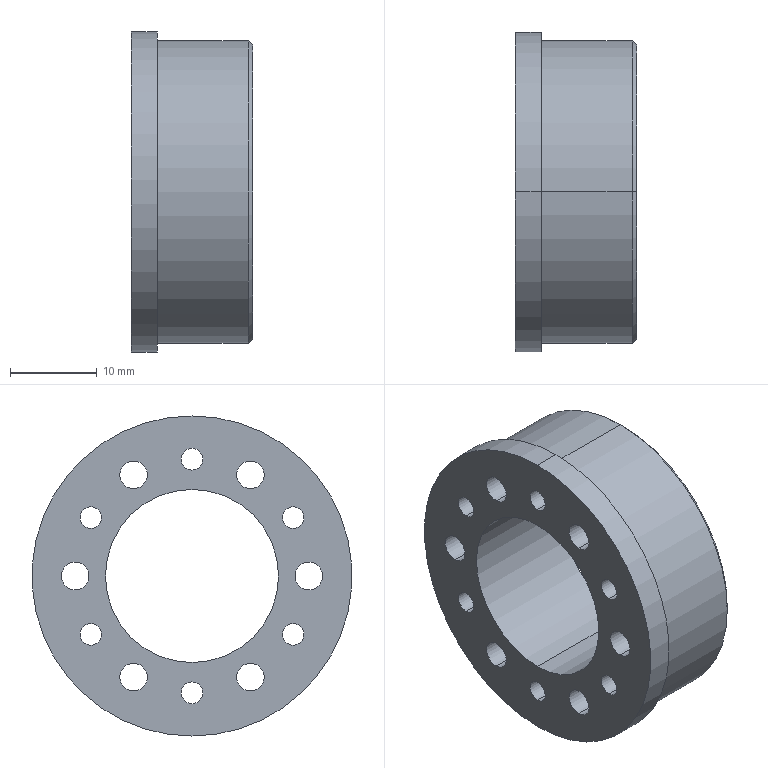Part | SolidWorks | features ICE 2, Chamfer 1, HoleWzd 1, Revolution 1 | 1 solid | 65 faces | box 14 x 37 x 37 mm | volume 7882 mm3 | cylinder 42 | cone 14 | plane 9 | commonest cylinder face diameters 2.5 x12 3.2 x12 6 x12 20 x2 35 x2 37 x2